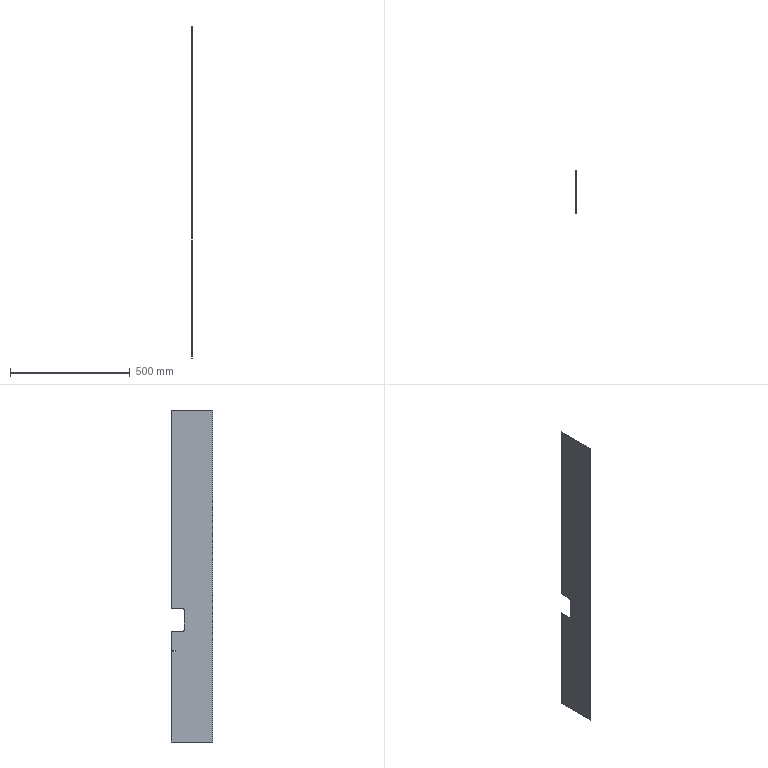Part | STEP file | Trunking 3 | 1 solid | 16 faces | box 1.5 x 173.707 x 1387 mm | volume 353324 mm3 | plane 14 | cylinder 2 | commonest cylinder face diameters 20 x2
STEP:
#1=CARTESIAN_POINT('',(-1.5,495.892,-105.329));
#2=VERTEX_POINT('',#1);
#3=CARTESIAN_POINT('',(-1.5,322.185,-105.329));
#4=VERTEX_POINT('',#3);
#5=CARTESIAN_POINT('',(-1.5,428.185,-105.329));
#6=DIRECTION('',(0.,-1.,0.));
#7=VECTOR('',#6,1000.);
#8=LINE('',#5,#7);
#9=EDGE_CURVE('',#2,#4,#8,.T.);
#10=ORIENTED_EDGE('',*,*,#9,.T.);
#11=CARTESIAN_POINT('',(-1.5,322.185,1281.931));
#12=VERTEX_POINT('',#11);
#13=CARTESIAN_POINT('',(-1.5,322.185,0.));
#14=DIRECTION('',(0.,0.,1.));
#15=VECTOR('',#14,1000.);
#16=LINE('',#13,#15);
#17=EDGE_CURVE('',#4,#12,#16,.T.);
#18=ORIENTED_EDGE('',*,*,#17,.T.);
#19=CARTESIAN_POINT('',(-1.5,495.892,1281.931));
#20=VERTEX_POINT('',#19);
#21=CARTESIAN_POINT('',(-1.5,428.185,1281.931));
#22=DIRECTION('',(0.,1.,0.));
#23=VECTOR('',#22,1000.);
#24=LINE('',#21,#23);
#25=EDGE_CURVE('',#12,#20,#24,.T.);
#26=ORIENTED_EDGE('',*,*,#25,.T.);
#27=CARTESIAN_POINT('',(-1.5,495.892,453.931));
#28=VERTEX_POINT('',#27);
#29=CARTESIAN_POINT('',(-1.5,495.892,0.));
#30=DIRECTION('',(0.,0.,-1.));
#31=VECTOR('',#30,1000.);
#32=LINE('',#29,#31);
#33=EDGE_CURVE('',#20,#28,#32,.T.);
#34=ORIENTED_EDGE('',*,*,#33,.T.);
#35=CARTESIAN_POINT('',(-1.5,450.892,453.931));
#36=VERTEX_POINT('',#35);
#37=CARTESIAN_POINT('',(-1.5,428.185,453.931));
#38=DIRECTION('',(0.,-1.,0.));
#39=VECTOR('',#38,1000.);
#40=LINE('',#37,#39);
#41=EDGE_CURVE('',#28,#36,#40,.T.);
#42=ORIENTED_EDGE('',*,*,#41,.T.);
#43=CARTESIAN_POINT('',(-1.5,440.892,443.931));
#44=VERTEX_POINT('',#43);
#45=CARTESIAN_POINT('',(-1.5,450.892,443.931));
#46=DIRECTION('',(1.,0.,0.));
#47=DIRECTION('',(0.,0.,-1.));
#48=AXIS2_PLACEMENT_3D('',#45,#46,#47);
#49=CIRCLE('',#48,10.);
#50=EDGE_CURVE('',#36,#44,#49,.T.);
#51=ORIENTED_EDGE('',*,*,#50,.T.);
#52=CARTESIAN_POINT('',(-1.5,440.892,365.931));
#53=VERTEX_POINT('',#52);
#54=CARTESIAN_POINT('',(-1.5,440.892,0.));
#55=DIRECTION('',(0.,0.,-1.));
#56=VECTOR('',#55,1000.);
#57=LINE('',#54,#56);
#58=EDGE_CURVE('',#44,#53,#57,.T.);
#59=ORIENTED_EDGE('',*,*,#58,.T.);
#60=CARTESIAN_POINT('',(-1.5,450.892,355.931));
#61=VERTEX_POINT('',#60);
#62=CARTESIAN_POINT('',(-1.5,450.892,365.931));
#63=DIRECTION('',(1.,0.,0.));
#64=DIRECTION('',(0.,0.,-1.));
#65=AXIS2_PLACEMENT_3D('',#62,#63,#64);
#66=CIRCLE('',#65,10.);
#67=EDGE_CURVE('',#53,#61,#66,.T.);
#68=ORIENTED_EDGE('',*,*,#67,.T.);
#69=CARTESIAN_POINT('',(-1.5,495.892,355.931));
#70=VERTEX_POINT('',#69);
#71=CARTESIAN_POINT('',(-1.5,428.185,355.931));
#72=DIRECTION('',(0.,1.,0.));
#73=VECTOR('',#72,1000.);
#74=LINE('',#71,#73);
#75=EDGE_CURVE('',#61,#70,#74,.T.);
#76=ORIENTED_EDGE('',*,*,#75,.T.);
#77=CARTESIAN_POINT('',(-1.5,495.892,275.931));
#78=VERTEX_POINT('',#77);
#79=CARTESIAN_POINT('',(-1.5,495.892,0.));
#80=DIRECTION('',(0.,0.,-1.));
#81=VECTOR('',#80,1000.);
#82=LINE('',#79,#81);
#83=EDGE_CURVE('',#70,#78,#82,.T.);
#84=ORIENTED_EDGE('',*,*,#83,.T.);
#85=CARTESIAN_POINT('',(-1.5,479.892,275.931));
#86=VERTEX_POINT('',#85);
#87=CARTESIAN_POINT('',(-1.5,428.185,275.931));
#88=DIRECTION('',(0.,-1.,0.));
#89=VECTOR('',#88,1000.);
#90=LINE('',#87,#89);
#91=EDGE_CURVE('',#78,#86,#90,.T.);
#92=ORIENTED_EDGE('',*,*,#91,.T.);
#93=CARTESIAN_POINT('',(-1.5,479.892,270.931));
#94=VERTEX_POINT('',#93);
#95=CARTESIAN_POINT('',(-1.5,479.892,0.));
#96=DIRECTION('',(0.,0.,-1.));
#97=VECTOR('',#96,1000.);
#98=LINE('',#95,#97);
#99=EDGE_CURVE('',#86,#94,#98,.T.);
#100=ORIENTED_EDGE('',*,*,#99,.T.);
#101=CARTESIAN_POINT('',(-1.5,495.892,270.931));
#102=VERTEX_POINT('',#101);
#103=CARTESIAN_POINT('',(-1.5,428.185,270.931));
#104=DIRECTION('',(0.,1.,0.));
#105=VECTOR('',#104,1000.);
#106=LINE('',#103,#105);
#107=EDGE_CURVE('',#94,#102,#106,.T.);
#108=ORIENTED_EDGE('',*,*,#107,.T.);
#109=CARTESIAN_POINT('',(-1.5,495.892,0.));
#110=DIRECTION('',(0.,0.,-1.));
#111=VECTOR('',#110,1000.);
#112=LINE('',#109,#111);
#113=EDGE_CURVE('',#102,#2,#112,.T.);
#114=ORIENTED_EDGE('',*,*,#113,.T.);
#115=EDGE_LOOP('',(#10,#18,#26,#34,#42,#51,#59,#68,#76,#84,#92,#100,#108,#114));
#116=FACE_OUTER_BOUND('',#115,.T.);
#117=CARTESIAN_POINT('',(-1.5,428.185,0.));
#118=DIRECTION('',(-1.,0.,0.));
#119=DIRECTION('',(0.,-1.,0.));
#120=AXIS2_PLACEMENT_3D('',#117,#118,#119);
#121=PLANE('',#120);
#122=ADVANCED_FACE('',(#116),#121,.T.);
#123=CARTESIAN_POINT('',(0.,322.185,-105.329));
#124=VERTEX_POINT('',#123);
#125=CARTESIAN_POINT('',(0.,322.185,-105.329));
#126=DIRECTION('',(-1.,0.,0.));
#127=VECTOR('',#126,1000.);
#128=LINE('',#125,#127);
#129=EDGE_CURVE('',#124,#4,#128,.T.);
#130=ORIENTED_EDGE('',*,*,#129,.F.);
#131=CARTESIAN_POINT('',(0.,322.185,1281.931));
#132=VERTEX_POINT('',#131);
#133=CARTESIAN_POINT('',(0.,322.185,-105.329));
#134=DIRECTION('',(0.,0.,-1.));
#135=VECTOR('',#134,1000.);
#136=LINE('',#133,#135);
#137=EDGE_CURVE('',#132,#124,#136,.T.);
#138=ORIENTED_EDGE('',*,*,#137,.F.);
#139=CARTESIAN_POINT('',(0.,322.185,1281.931));
#140=DIRECTION('',(1.,0.,0.));
#141=VECTOR('',#140,1000.);
#142=LINE('',#139,#141);
#143=EDGE_CURVE('',#12,#132,#142,.T.);
#144=ORIENTED_EDGE('',*,*,#143,.F.);
#145=ORIENTED_EDGE('',*,*,#17,.F.);
#146=EDGE_LOOP('',(#130,#138,#144,#145));
#147=FACE_OUTER_BOUND('',#146,.T.);
#148=CARTESIAN_POINT('',(0.,322.185,-105.329));
#149=DIRECTION('',(0.,1.,0.));
#150=DIRECTION('',(-1.,0.,0.));
#151=AXIS2_PLACEMENT_3D('',#148,#149,#150);
#152=PLANE('',#151);
#153=ADVANCED_FACE('',(#147),#152,.F.);
#154=CARTESIAN_POINT('',(0.,495.892,-105.329));
#155=VERTEX_POINT('',#154);
#156=CARTESIAN_POINT('',(0.,495.892,-105.329));
#157=DIRECTION('',(-1.,0.,0.));
#158=VECTOR('',#157,1000.);
#159=LINE('',#156,#158);
#160=EDGE_CURVE('',#155,#2,#159,.T.);
#161=ORIENTED_EDGE('',*,*,#160,.F.);
#162=CARTESIAN_POINT('',(0.,426.685,-105.329));
#163=DIRECTION('',(0.,1.,0.));
#164=VECTOR('',#163,1000.);
#165=LINE('',#162,#164);
#166=EDGE_CURVE('',#124,#155,#165,.T.);
#167=ORIENTED_EDGE('',*,*,#166,.F.);
#168=ORIENTED_EDGE('',*,*,#129,.T.);
#169=ORIENTED_EDGE('',*,*,#9,.F.);
#170=EDGE_LOOP('',(#161,#167,#168,#169));
#171=FACE_OUTER_BOUND('',#170,.T.);
#172=CARTESIAN_POINT('',(0.,426.685,-105.329));
#173=DIRECTION('',(0.,0.,1.));
#174=DIRECTION('',(0.,-1.,0.));
#175=AXIS2_PLACEMENT_3D('',#172,#173,#174);
#176=PLANE('',#175);
#177=ADVANCED_FACE('',(#171),#176,.F.);
#178=ORIENTED_EDGE('',*,*,#160,.T.);
#179=ORIENTED_EDGE('',*,*,#113,.F.);
#180=CARTESIAN_POINT('',(0.,495.892,270.931));
#181=VERTEX_POINT('',#180);
#182=CARTESIAN_POINT('',(-1.5,495.892,270.931));
#183=DIRECTION('',(1.,0.,0.));
#184=VECTOR('',#183,1000.);
#185=LINE('',#182,#184);
#186=EDGE_CURVE('',#102,#181,#185,.T.);
#187=ORIENTED_EDGE('',*,*,#186,.T.);
#188=CARTESIAN_POINT('',(0.,495.892,1281.931));
#189=DIRECTION('',(0.,0.,-1.));
#190=VECTOR('',#189,1000.);
#191=LINE('',#188,#190);
#192=EDGE_CURVE('',#181,#155,#191,.T.);
#193=ORIENTED_EDGE('',*,*,#192,.T.);
#194=EDGE_LOOP('',(#178,#179,#187,#193));
#195=FACE_OUTER_BOUND('',#194,.T.);
#196=CARTESIAN_POINT('',(-1.5,495.892,1281.931));
#197=DIRECTION('',(0.,1.,0.));
#198=DIRECTION('',(0.,0.,1.));
#199=AXIS2_PLACEMENT_3D('',#196,#197,#198);
#200=PLANE('',#199);
#201=ADVANCED_FACE('',(#195),#200,.T.);
#202=CARTESIAN_POINT('',(0.,479.892,270.931));
#203=VERTEX_POINT('',#202);
#204=CARTESIAN_POINT('',(-10.,479.892,270.931));
#205=DIRECTION('',(-1.,0.,0.));
#206=VECTOR('',#205,1000.);
#207=LINE('',#204,#206);
#208=EDGE_CURVE('',#203,#94,#207,.T.);
#209=ORIENTED_EDGE('',*,*,#208,.F.);
#210=CARTESIAN_POINT('',(0.,495.892,270.931));
#211=DIRECTION('',(0.,-1.,0.));
#212=VECTOR('',#211,1000.);
#213=LINE('',#210,#212);
#214=EDGE_CURVE('',#181,#203,#213,.T.);
#215=ORIENTED_EDGE('',*,*,#214,.F.);
#216=ORIENTED_EDGE('',*,*,#186,.F.);
#217=ORIENTED_EDGE('',*,*,#107,.F.);
#218=EDGE_LOOP('',(#209,#215,#216,#217));
#219=FACE_OUTER_BOUND('',#218,.T.);
#220=CARTESIAN_POINT('',(-10.,495.892,270.931));
#221=DIRECTION('',(0.,0.,-1.));
#222=DIRECTION('',(-1.,0.,0.));
#223=AXIS2_PLACEMENT_3D('',#220,#221,#222);
#224=PLANE('',#223);
#225=ADVANCED_FACE('',(#219),#224,.F.);
#226=CARTESIAN_POINT('',(0.,479.892,275.931));
#227=VERTEX_POINT('',#226);
#228=CARTESIAN_POINT('',(-10.,479.892,275.931));
#229=DIRECTION('',(-1.,0.,0.));
#230=VECTOR('',#229,1000.);
#231=LINE('',#228,#230);
#232=EDGE_CURVE('',#227,#86,#231,.T.);
#233=ORIENTED_EDGE('',*,*,#232,.F.);
#234=CARTESIAN_POINT('',(0.,479.892,275.931));
#235=DIRECTION('',(0.,0.,1.));
#236=VECTOR('',#235,1000.);
#237=LINE('',#234,#236);
#238=EDGE_CURVE('',#203,#227,#237,.T.);
#239=ORIENTED_EDGE('',*,*,#238,.F.);
#240=ORIENTED_EDGE('',*,*,#208,.T.);
#241=ORIENTED_EDGE('',*,*,#99,.F.);
#242=EDGE_LOOP('',(#233,#239,#240,#241));
#243=FACE_OUTER_BOUND('',#242,.T.);
#244=CARTESIAN_POINT('',(-10.,479.892,275.931));
#245=DIRECTION('',(0.,-1.,0.));
#246=DIRECTION('',(0.,0.,-1.));
#247=AXIS2_PLACEMENT_3D('',#244,#245,#246);
#248=PLANE('',#247);
#249=ADVANCED_FACE('',(#243),#248,.F.);
#250=CARTESIAN_POINT('',(0.,495.892,275.931));
#251=VERTEX_POINT('',#250);
#252=CARTESIAN_POINT('',(-10.,495.892,275.931));
#253=DIRECTION('',(-1.,0.,0.));
#254=VECTOR('',#253,1000.);
#255=LINE('',#252,#254);
#256=EDGE_CURVE('',#251,#78,#255,.T.);
#257=ORIENTED_EDGE('',*,*,#256,.F.);
#258=CARTESIAN_POINT('',(0.,495.892,275.931));
#259=DIRECTION('',(0.,1.,0.));
#260=VECTOR('',#259,1000.);
#261=LINE('',#258,#260);
#262=EDGE_CURVE('',#227,#251,#261,.T.);
#263=ORIENTED_EDGE('',*,*,#262,.F.);
#264=ORIENTED_EDGE('',*,*,#232,.T.);
#265=ORIENTED_EDGE('',*,*,#91,.F.);
#266=EDGE_LOOP('',(#257,#263,#264,#265));
#267=FACE_OUTER_BOUND('',#266,.T.);
#268=CARTESIAN_POINT('',(-10.,495.892,275.931));
#269=DIRECTION('',(0.,0.,1.));
#270=DIRECTION('',(1.,0.,0.));
#271=AXIS2_PLACEMENT_3D('',#268,#269,#270);
#272=PLANE('',#271);
#273=ADVANCED_FACE('',(#267),#272,.F.);
#274=ORIENTED_EDGE('',*,*,#256,.T.);
#275=ORIENTED_EDGE('',*,*,#83,.F.);
#276=CARTESIAN_POINT('',(0.,495.892,355.931));
#277=VERTEX_POINT('',#276);
#278=CARTESIAN_POINT('',(-1.5,495.892,355.931));
#279=DIRECTION('',(1.,0.,0.));
#280=VECTOR('',#279,1000.);
#281=LINE('',#278,#280);
#282=EDGE_CURVE('',#70,#277,#281,.T.);
#283=ORIENTED_EDGE('',*,*,#282,.T.);
#284=CARTESIAN_POINT('',(0.,495.892,1281.931));
#285=DIRECTION('',(0.,0.,-1.));
#286=VECTOR('',#285,1000.);
#287=LINE('',#284,#286);
#288=EDGE_CURVE('',#277,#251,#287,.T.);
#289=ORIENTED_EDGE('',*,*,#288,.T.);
#290=EDGE_LOOP('',(#274,#275,#283,#289));
#291=FACE_OUTER_BOUND('',#290,.T.);
#292=CARTESIAN_POINT('',(-1.5,495.892,1281.931));
#293=DIRECTION('',(0.,1.,0.));
#294=DIRECTION('',(0.,0.,1.));
#295=AXIS2_PLACEMENT_3D('',#292,#293,#294);
#296=PLANE('',#295);
#297=ADVANCED_FACE('',(#291),#296,.T.);
#298=CARTESIAN_POINT('',(0.,450.892,355.931));
#299=VERTEX_POINT('',#298);
#300=CARTESIAN_POINT('',(-10.,450.892,355.931));
#301=DIRECTION('',(-1.,0.,0.));
#302=VECTOR('',#301,1000.);
#303=LINE('',#300,#302);
#304=EDGE_CURVE('',#299,#61,#303,.T.);
#305=ORIENTED_EDGE('',*,*,#304,.F.);
#306=CARTESIAN_POINT('',(0.,495.892,355.931));
#307=DIRECTION('',(0.,-1.,0.));
#308=VECTOR('',#307,1000.);
#309=LINE('',#306,#308);
#310=EDGE_CURVE('',#277,#299,#309,.T.);
#311=ORIENTED_EDGE('',*,*,#310,.F.);
#312=ORIENTED_EDGE('',*,*,#282,.F.);
#313=ORIENTED_EDGE('',*,*,#75,.F.);
#314=EDGE_LOOP('',(#305,#311,#312,#313));
#315=FACE_OUTER_BOUND('',#314,.T.);
#316=CARTESIAN_POINT('',(-10.,495.892,355.931));
#317=DIRECTION('',(0.,0.,-1.));
#318=DIRECTION('',(0.,1.,0.));
#319=AXIS2_PLACEMENT_3D('',#316,#317,#318);
#320=PLANE('',#319);
#321=ADVANCED_FACE('',(#315),#320,.F.);
#322=CARTESIAN_POINT('',(0.,440.892,365.931));
#323=VERTEX_POINT('',#322);
#324=CARTESIAN_POINT('',(-10.,440.892,365.931));
#325=DIRECTION('',(-1.,0.,0.));
#326=VECTOR('',#325,1000.);
#327=LINE('',#324,#326);
#328=EDGE_CURVE('',#323,#53,#327,.T.);
#329=ORIENTED_EDGE('',*,*,#328,.F.);
#330=CARTESIAN_POINT('',(0.,450.892,365.931));
#331=DIRECTION('',(-1.,0.,0.));
#332=DIRECTION('',(0.,0.,-1.));
#333=AXIS2_PLACEMENT_3D('',#330,#331,#332);
#334=CIRCLE('',#333,10.);
#335=EDGE_CURVE('',#299,#323,#334,.T.);
#336=ORIENTED_EDGE('',*,*,#335,.F.);
#337=ORIENTED_EDGE('',*,*,#304,.T.);
#338=ORIENTED_EDGE('',*,*,#67,.F.);
#339=EDGE_LOOP('',(#329,#336,#337,#338));
#340=FACE_OUTER_BOUND('',#339,.T.);
#341=CARTESIAN_POINT('',(-10.,450.892,365.931));
#342=DIRECTION('',(1.,0.,0.));
#343=DIRECTION('',(0.,0.,-1.));
#344=AXIS2_PLACEMENT_3D('',#341,#342,#343);
#345=CYLINDRICAL_SURFACE('',#344,10.);
#346=ADVANCED_FACE('',(#340),#345,.F.);
#347=CARTESIAN_POINT('',(0.,440.892,443.931));
#348=VERTEX_POINT('',#347);
#349=CARTESIAN_POINT('',(-10.,440.892,443.931));
#350=DIRECTION('',(-1.,0.,0.));
#351=VECTOR('',#350,1000.);
#352=LINE('',#349,#351);
#353=EDGE_CURVE('',#348,#44,#352,.T.);
#354=ORIENTED_EDGE('',*,*,#353,.F.);
#355=CARTESIAN_POINT('',(0.,440.892,443.931));
#356=DIRECTION('',(0.,0.,1.));
#357=VECTOR('',#356,1000.);
#358=LINE('',#355,#357);
#359=EDGE_CURVE('',#323,#348,#358,.T.);
#360=ORIENTED_EDGE('',*,*,#359,.F.);
#361=ORIENTED_EDGE('',*,*,#328,.T.);
#362=ORIENTED_EDGE('',*,*,#58,.F.);
#363=EDGE_LOOP('',(#354,#360,#361,#362));
#364=FACE_OUTER_BOUND('',#363,.T.);
#365=CARTESIAN_POINT('',(-10.,440.892,443.931));
#366=DIRECTION('',(0.,-1.,0.));
#367=DIRECTION('',(0.,0.,-1.));
#368=AXIS2_PLACEMENT_3D('',#365,#366,#367);
#369=PLANE('',#368);
#370=ADVANCED_FACE('',(#364),#369,.F.);
#371=CARTESIAN_POINT('',(0.,450.892,453.931));
#372=VERTEX_POINT('',#371);
#373=CARTESIAN_POINT('',(-10.,450.892,453.931));
#374=DIRECTION('',(-1.,0.,0.));
#375=VECTOR('',#374,1000.);
#376=LINE('',#373,#375);
#377=EDGE_CURVE('',#372,#36,#376,.T.);
#378=ORIENTED_EDGE('',*,*,#377,.F.);
#379=CARTESIAN_POINT('',(0.,450.892,443.931));
#380=DIRECTION('',(-1.,0.,0.));
#381=DIRECTION('',(0.,0.,-1.));
#382=AXIS2_PLACEMENT_3D('',#379,#380,#381);
#383=CIRCLE('',#382,10.);
#384=EDGE_CURVE('',#348,#372,#383,.T.);
#385=ORIENTED_EDGE('',*,*,#384,.F.);
#386=ORIENTED_EDGE('',*,*,#353,.T.);
#387=ORIENTED_EDGE('',*,*,#50,.F.);
#388=EDGE_LOOP('',(#378,#385,#386,#387));
#389=FACE_OUTER_BOUND('',#388,.T.);
#390=CARTESIAN_POINT('',(-10.,450.892,443.931));
#391=DIRECTION('',(1.,0.,0.));
#392=DIRECTION('',(0.,0.,-1.));
#393=AXIS2_PLACEMENT_3D('',#390,#391,#392);
#394=CYLINDRICAL_SURFACE('',#393,10.);
#395=ADVANCED_FACE('',(#389),#394,.F.);
#396=CARTESIAN_POINT('',(0.,495.892,453.931));
#397=VERTEX_POINT('',#396);
#398=CARTESIAN_POINT('',(-10.,495.892,453.931));
#399=DIRECTION('',(-1.,0.,0.));
#400=VECTOR('',#399,1000.);
#401=LINE('',#398,#400);
#402=EDGE_CURVE('',#397,#28,#401,.T.);
#403=ORIENTED_EDGE('',*,*,#402,.F.);
#404=CARTESIAN_POINT('',(0.,495.892,453.931));
#405=DIRECTION('',(0.,1.,0.));
#406=VECTOR('',#405,1000.);
#407=LINE('',#404,#406);
#408=EDGE_CURVE('',#372,#397,#407,.T.);
#409=ORIENTED_EDGE('',*,*,#408,.F.);
#410=ORIENTED_EDGE('',*,*,#377,.T.);
#411=ORIENTED_EDGE('',*,*,#41,.F.);
#412=EDGE_LOOP('',(#403,#409,#410,#411));
#413=FACE_OUTER_BOUND('',#412,.T.);
#414=CARTESIAN_POINT('',(-10.,495.892,453.931));
#415=DIRECTION('',(0.,0.,1.));
#416=DIRECTION('',(0.,-1.,0.));
#417=AXIS2_PLACEMENT_3D('',#414,#415,#416);
#418=PLANE('',#417);
#419=ADVANCED_FACE('',(#413),#418,.F.);
#420=CARTESIAN_POINT('',(0.,495.892,1281.931));
#421=VERTEX_POINT('',#420);
#422=CARTESIAN_POINT('',(-1.5,495.892,1281.931));
#423=DIRECTION('',(1.,0.,0.));
#424=VECTOR('',#423,1000.);
#425=LINE('',#422,#424);
#426=EDGE_CURVE('',#20,#421,#425,.T.);
#427=ORIENTED_EDGE('',*,*,#426,.T.);
#428=CARTESIAN_POINT('',(0.,495.892,1281.931));
#429=DIRECTION('',(0.,0.,-1.));
#430=VECTOR('',#429,1000.);
#431=LINE('',#428,#430);
#432=EDGE_CURVE('',#421,#397,#431,.T.);
#433=ORIENTED_EDGE('',*,*,#432,.T.);
#434=ORIENTED_EDGE('',*,*,#402,.T.);
#435=ORIENTED_EDGE('',*,*,#33,.F.);
#436=EDGE_LOOP('',(#427,#433,#434,#435));
#437=FACE_OUTER_BOUND('',#436,.T.);
#438=CARTESIAN_POINT('',(-1.5,495.892,1281.931));
#439=DIRECTION('',(0.,1.,0.));
#440=DIRECTION('',(0.,0.,1.));
#441=AXIS2_PLACEMENT_3D('',#438,#439,#440);
#442=PLANE('',#441);
#443=ADVANCED_FACE('',(#437),#442,.T.);
#444=ORIENTED_EDGE('',*,*,#426,.F.);
#445=ORIENTED_EDGE('',*,*,#25,.F.);
#446=ORIENTED_EDGE('',*,*,#143,.T.);
#447=CARTESIAN_POINT('',(0.,322.185,1281.931));
#448=DIRECTION('',(0.,-1.,0.));
#449=VECTOR('',#448,1000.);
#450=LINE('',#447,#449);
#451=EDGE_CURVE('',#421,#132,#450,.T.);
#452=ORIENTED_EDGE('',*,*,#451,.F.);
#453=EDGE_LOOP('',(#444,#445,#446,#452));
#454=FACE_OUTER_BOUND('',#453,.T.);
#455=CARTESIAN_POINT('',(0.,322.185,1281.931));
#456=DIRECTION('',(0.,0.,-1.));
#457=DIRECTION('',(-1.,0.,0.));
#458=AXIS2_PLACEMENT_3D('',#455,#456,#457);
#459=PLANE('',#458);
#460=ADVANCED_FACE('',(#454),#459,.F.);
#461=ORIENTED_EDGE('',*,*,#192,.F.);
#462=ORIENTED_EDGE('',*,*,#214,.T.);
#463=ORIENTED_EDGE('',*,*,#238,.T.);
#464=ORIENTED_EDGE('',*,*,#262,.T.);
#465=ORIENTED_EDGE('',*,*,#288,.F.);
#466=ORIENTED_EDGE('',*,*,#310,.T.);
#467=ORIENTED_EDGE('',*,*,#335,.T.);
#468=ORIENTED_EDGE('',*,*,#359,.T.);
#469=ORIENTED_EDGE('',*,*,#384,.T.);
#470=ORIENTED_EDGE('',*,*,#408,.T.);
#471=ORIENTED_EDGE('',*,*,#432,.F.);
#472=ORIENTED_EDGE('',*,*,#451,.T.);
#473=ORIENTED_EDGE('',*,*,#137,.T.);
#474=ORIENTED_EDGE('',*,*,#166,.T.);
#475=EDGE_LOOP('',(#461,#462,#463,#464,#465,#466,#467,#468,#469,#470,#471,#472,#473,#474));
#476=FACE_OUTER_BOUND('',#475,.T.);
#477=CARTESIAN_POINT('',(0.,0.,0.));
#478=DIRECTION('',(-1.,0.,0.));
#479=DIRECTION('',(0.,0.,1.));
#480=AXIS2_PLACEMENT_3D('',#477,#478,#479);
#481=PLANE('',#480);
#482=ADVANCED_FACE('',(#476),#481,.F.);
#483=CLOSED_SHELL('',(#122,#153,#177,#201,#225,#249,#273,#297,#321,#346,#370,#395,#419,#443,#460,#482));
#484=MANIFOLD_SOLID_BREP('',#483);
#485=CARTESIAN_POINT('',(0.,0.,0.));
#486=DIRECTION('',(0.,0.,1.));
#487=DIRECTION('',(1.,0.,0.));
#488=AXIS2_PLACEMENT_3D('',#485,#486,#487);
#489=(LENGTH_UNIT()NAMED_UNIT(*)SI_UNIT(.MILLI.,.METRE.));
#490=UNCERTAINTY_MEASURE_WITH_UNIT(LENGTH_MEASURE(0.00001),#489,'','');
#491=(NAMED_UNIT(*)PLANE_ANGLE_UNIT()SI_UNIT($,.RADIAN.));
#492=(NAMED_UNIT(*)SI_UNIT($,.STERADIAN.)SOLID_ANGLE_UNIT());
#493=(GEOMETRIC_REPRESENTATION_CONTEXT(3)GLOBAL_UNCERTAINTY_ASSIGNED_CONTEXT((#490))GLOBAL_UNIT_ASSIGNED_CONTEXT((#489,#491,#492))REPRESENTATION_CONTEXT('',''));
#494=ADVANCED_BREP_SHAPE_REPRESENTATION('',(#484,#488),#493);